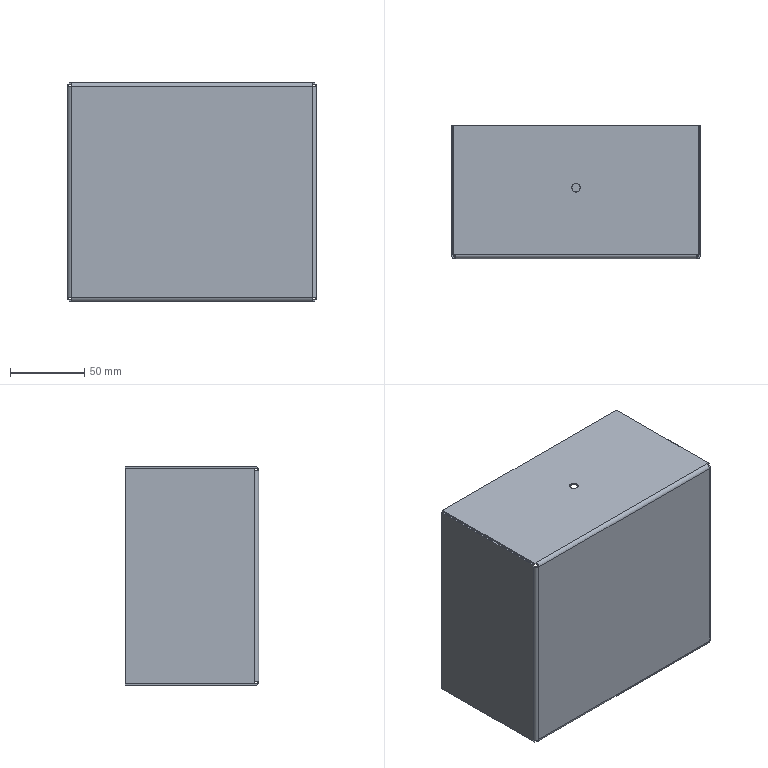Part | NX | 1 solid | 50 faces | box 167.7 x 90 x 147.4 mm | volume 79424 mm3 | plane 38 | cylinder 10 | cone 2 | commonest cylinder face diameters 3.2 x4 5.2 x4 5.5 x2
STEP:
#1=CARTESIAN_POINT('',(2221.7,-122.9,209.129));
#2=VERTEX_POINT('',#1);
#3=CARTESIAN_POINT('',(2221.7,-35.5,209.129));
#4=VERTEX_POINT('',#3);
#5=CARTESIAN_POINT('',(2221.7,-124.5,209.129));
#6=DIRECTION('',(0.,1.,0.));
#7=VECTOR('',#6,1000.);
#8=LINE('',#5,#7);
#9=EDGE_CURVE('',#2,#4,#8,.T.);
#10=ORIENTED_EDGE('',*,*,#9,.F.);
#11=CARTESIAN_POINT('',(2221.7,-122.9,207.6));
#12=VERTEX_POINT('',#11);
#13=CARTESIAN_POINT('',(2221.7,-122.9,119.504));
#14=DIRECTION('',(0.,0.,1.));
#15=VECTOR('',#14,1000.);
#16=LINE('',#13,#15);
#17=EDGE_CURVE('',#12,#2,#16,.T.);
#18=ORIENTED_EDGE('',*,*,#17,.F.);
#19=CARTESIAN_POINT('',(2221.7,-122.9,65.4));
#20=VERTEX_POINT('',#19);
#21=CARTESIAN_POINT('',(2221.7,-122.9,119.504));
#22=DIRECTION('',(0.,0.,1.));
#23=VECTOR('',#22,1000.);
#24=LINE('',#21,#23);
#25=EDGE_CURVE('',#20,#12,#24,.T.);
#26=ORIENTED_EDGE('',*,*,#25,.F.);
#27=CARTESIAN_POINT('',(2221.7,-122.9,63.871));
#28=VERTEX_POINT('',#27);
#29=CARTESIAN_POINT('',(2221.7,-122.9,119.504));
#30=DIRECTION('',(0.,0.,1.));
#31=VECTOR('',#30,1000.);
#32=LINE('',#29,#31);
#33=EDGE_CURVE('',#28,#20,#32,.T.);
#34=ORIENTED_EDGE('',*,*,#33,.F.);
#35=CARTESIAN_POINT('',(2221.7,-35.5,63.871));
#36=VERTEX_POINT('',#35);
#37=CARTESIAN_POINT('',(2221.7,-124.5,63.871));
#38=DIRECTION('',(0.,-1.,0.));
#39=VECTOR('',#38,1000.);
#40=LINE('',#37,#39);
#41=EDGE_CURVE('',#36,#28,#40,.T.);
#42=ORIENTED_EDGE('',*,*,#41,.F.);
#43=CARTESIAN_POINT('',(2221.7,-35.5,119.504));
#44=DIRECTION('',(0.,0.,-1.));
#45=VECTOR('',#44,1000.);
#46=LINE('',#43,#45);
#47=EDGE_CURVE('',#4,#36,#46,.T.);
#48=ORIENTED_EDGE('',*,*,#47,.F.);
#49=EDGE_LOOP('',(#10,#18,#26,#34,#42,#48));
#50=FACE_BOUND('',#49,.T.);
#51=CARTESIAN_POINT('',(2221.7,-188.294,119.504));
#52=DIRECTION('',(-1.,0.,0.));
#53=DIRECTION('',(0.,0.,1.));
#54=AXIS2_PLACEMENT_3D('',#51,#52,#53);
#55=PLANE('',#54);
#56=ADVANCED_FACE('',(#50),#55,.F.);
#57=CARTESIAN_POINT('',(2056.6,-122.9,62.8));
#58=VERTEX_POINT('',#57);
#59=CARTESIAN_POINT('',(2219.1,-122.9,62.8));
#60=VERTEX_POINT('',#59);
#61=CARTESIAN_POINT('',(2156.806,-122.9,62.8));
#62=DIRECTION('',(1.,0.,0.));
#63=VECTOR('',#62,1000.);
#64=LINE('',#61,#63);
#65=EDGE_CURVE('',#58,#60,#64,.T.);
#66=ORIENTED_EDGE('',*,*,#65,.F.);
#67=CARTESIAN_POINT('',(2055.071,-122.9,62.8));
#68=VERTEX_POINT('',#67);
#69=CARTESIAN_POINT('',(2156.806,-122.9,62.8));
#70=DIRECTION('',(1.,0.,0.));
#71=VECTOR('',#70,1000.);
#72=LINE('',#69,#71);
#73=EDGE_CURVE('',#68,#58,#72,.T.);
#74=ORIENTED_EDGE('',*,*,#73,.F.);
#75=CARTESIAN_POINT('',(2055.071,-35.5,62.8));
#76=VERTEX_POINT('',#75);
#77=CARTESIAN_POINT('',(2055.071,-124.5,62.8));
#78=DIRECTION('',(0.,-1.,0.));
#79=VECTOR('',#78,1000.);
#80=LINE('',#77,#79);
#81=EDGE_CURVE('',#76,#68,#80,.T.);
#82=ORIENTED_EDGE('',*,*,#81,.F.);
#83=CARTESIAN_POINT('',(2220.629,-35.5,62.8));
#84=VERTEX_POINT('',#83);
#85=CARTESIAN_POINT('',(2156.806,-35.5,62.8));
#86=DIRECTION('',(-1.,0.,0.));
#87=VECTOR('',#86,1000.);
#88=LINE('',#85,#87);
#89=EDGE_CURVE('',#84,#76,#88,.T.);
#90=ORIENTED_EDGE('',*,*,#89,.F.);
#91=CARTESIAN_POINT('',(2220.629,-122.9,62.8));
#92=VERTEX_POINT('',#91);
#93=CARTESIAN_POINT('',(2220.629,-124.5,62.8));
#94=DIRECTION('',(0.,1.,0.));
#95=VECTOR('',#94,1000.);
#96=LINE('',#93,#95);
#97=EDGE_CURVE('',#92,#84,#96,.T.);
#98=ORIENTED_EDGE('',*,*,#97,.F.);
#99=CARTESIAN_POINT('',(2156.806,-122.9,62.8));
#100=DIRECTION('',(1.,0.,0.));
#101=VECTOR('',#100,1000.);
#102=LINE('',#99,#101);
#103=EDGE_CURVE('',#60,#92,#102,.T.);
#104=ORIENTED_EDGE('',*,*,#103,.F.);
#105=EDGE_LOOP('',(#66,#74,#82,#90,#98,#104));
#106=FACE_BOUND('',#105,.T.);
#107=CARTESIAN_POINT('',(2156.806,-180.104,62.8));
#108=DIRECTION('',(0.,0.,1.));
#109=DIRECTION('',(1.,0.,0.));
#110=AXIS2_PLACEMENT_3D('',#107,#108,#109);
#111=PLANE('',#110);
#112=ADVANCED_FACE('',(#106),#111,.F.);
#113=CARTESIAN_POINT('',(2219.1,-125.5,207.6));
#114=VERTEX_POINT('',#113);
#115=CARTESIAN_POINT('',(2219.1,-122.9,207.6));
#116=DIRECTION('',(0.,0.,-1.));
#117=DIRECTION('',(1.,0.,0.));
#118=AXIS2_PLACEMENT_3D('',#115,#116,#117);
#119=CIRCLE('',#118,2.6);
#120=EDGE_CURVE('',#12,#114,#119,.T.);
#121=ORIENTED_EDGE('',*,*,#120,.T.);
#122=CARTESIAN_POINT('',(2219.1,-125.5,65.4));
#123=VERTEX_POINT('',#122);
#124=CARTESIAN_POINT('',(2219.1,-125.5,119.504));
#125=DIRECTION('',(0.,0.,1.));
#126=VECTOR('',#125,1000.);
#127=LINE('',#124,#126);
#128=EDGE_CURVE('',#123,#114,#127,.T.);
#129=ORIENTED_EDGE('',*,*,#128,.F.);
#130=CARTESIAN_POINT('',(2219.1,-122.9,65.4));
#131=DIRECTION('',(0.,0.,1.));
#132=DIRECTION('',(0.,-1.,0.));
#133=AXIS2_PLACEMENT_3D('',#130,#131,#132);
#134=CIRCLE('',#133,2.6);
#135=EDGE_CURVE('',#123,#20,#134,.T.);
#136=ORIENTED_EDGE('',*,*,#135,.T.);
#137=ORIENTED_EDGE('',*,*,#25,.T.);
#138=EDGE_LOOP('',(#121,#129,#136,#137));
#139=FACE_BOUND('',#138,.T.);
#140=CARTESIAN_POINT('',(2219.1,-122.9,65.4));
#141=DIRECTION('',(0.,0.,-1.));
#142=DIRECTION('',(1.,0.,0.));
#143=AXIS2_PLACEMENT_3D('',#140,#141,#142);
#144=CYLINDRICAL_SURFACE('',#143,2.6);
#145=ADVANCED_FACE('',(#139),#144,.T.);
#146=CARTESIAN_POINT('',(2054.,-122.9,65.4));
#147=VERTEX_POINT('',#146);
#148=CARTESIAN_POINT('',(2056.6,-125.5,65.4));
#149=VERTEX_POINT('',#148);
#150=CARTESIAN_POINT('',(2056.6,-122.9,65.4));
#151=DIRECTION('',(0.,0.,1.));
#152=DIRECTION('',(-1.,0.,0.));
#153=AXIS2_PLACEMENT_3D('',#150,#151,#152);
#154=CIRCLE('',#153,2.6);
#155=EDGE_CURVE('',#147,#149,#154,.T.);
#156=ORIENTED_EDGE('',*,*,#155,.T.);
#157=CARTESIAN_POINT('',(2056.6,-125.5,207.6));
#158=VERTEX_POINT('',#157);
#159=CARTESIAN_POINT('',(2056.6,-125.5,119.504));
#160=DIRECTION('',(0.,0.,-1.));
#161=VECTOR('',#160,1000.);
#162=LINE('',#159,#161);
#163=EDGE_CURVE('',#158,#149,#162,.T.);
#164=ORIENTED_EDGE('',*,*,#163,.F.);
#165=CARTESIAN_POINT('',(2054.,-122.9,207.6));
#166=VERTEX_POINT('',#165);
#167=CARTESIAN_POINT('',(2056.6,-122.9,207.6));
#168=DIRECTION('',(0.,0.,-1.));
#169=DIRECTION('',(0.,-1.,0.));
#170=AXIS2_PLACEMENT_3D('',#167,#168,#169);
#171=CIRCLE('',#170,2.6);
#172=EDGE_CURVE('',#158,#166,#171,.T.);
#173=ORIENTED_EDGE('',*,*,#172,.T.);
#174=CARTESIAN_POINT('',(2054.,-122.9,119.504));
#175=DIRECTION('',(0.,0.,-1.));
#176=VECTOR('',#175,1000.);
#177=LINE('',#174,#176);
#178=EDGE_CURVE('',#166,#147,#177,.T.);
#179=ORIENTED_EDGE('',*,*,#178,.T.);
#180=EDGE_LOOP('',(#156,#164,#173,#179));
#181=FACE_BOUND('',#180,.T.);
#182=CARTESIAN_POINT('',(2056.6,-122.9,207.6));
#183=DIRECTION('',(0.,0.,1.));
#184=DIRECTION('',(-1.,0.,0.));
#185=AXIS2_PLACEMENT_3D('',#182,#183,#184);
#186=CYLINDRICAL_SURFACE('',#185,2.6);
#187=ADVANCED_FACE('',(#181),#186,.T.);
#188=CARTESIAN_POINT('',(2054.,-122.9,63.871));
#189=VERTEX_POINT('',#188);
#190=CARTESIAN_POINT('',(2054.,-122.9,119.504));
#191=DIRECTION('',(0.,0.,1.));
#192=VECTOR('',#191,1000.);
#193=LINE('',#190,#192);
#194=EDGE_CURVE('',#189,#147,#193,.T.);
#195=ORIENTED_EDGE('',*,*,#194,.T.);
#196=ORIENTED_EDGE('',*,*,#178,.F.);
#197=CARTESIAN_POINT('',(2054.,-122.9,209.129));
#198=VERTEX_POINT('',#197);
#199=CARTESIAN_POINT('',(2054.,-122.9,119.504));
#200=DIRECTION('',(0.,0.,1.));
#201=VECTOR('',#200,1000.);
#202=LINE('',#199,#201);
#203=EDGE_CURVE('',#166,#198,#202,.T.);
#204=ORIENTED_EDGE('',*,*,#203,.T.);
#205=CARTESIAN_POINT('',(2054.,-35.5,209.129));
#206=VERTEX_POINT('',#205);
#207=CARTESIAN_POINT('',(2054.,-124.5,209.129));
#208=DIRECTION('',(0.,-1.,0.));
#209=VECTOR('',#208,1000.);
#210=LINE('',#207,#209);
#211=EDGE_CURVE('',#206,#198,#210,.T.);
#212=ORIENTED_EDGE('',*,*,#211,.F.);
#213=CARTESIAN_POINT('',(2054.,-35.5,63.871));
#214=VERTEX_POINT('',#213);
#215=CARTESIAN_POINT('',(2054.,-35.5,119.504));
#216=DIRECTION('',(0.,0.,1.));
#217=VECTOR('',#216,1000.);
#218=LINE('',#215,#217);
#219=EDGE_CURVE('',#214,#206,#218,.T.);
#220=ORIENTED_EDGE('',*,*,#219,.F.);
#221=CARTESIAN_POINT('',(2054.,-124.5,63.871));
#222=DIRECTION('',(0.,1.,0.));
#223=VECTOR('',#222,1000.);
#224=LINE('',#221,#223);
#225=EDGE_CURVE('',#189,#214,#224,.T.);
#226=ORIENTED_EDGE('',*,*,#225,.F.);
#227=EDGE_LOOP('',(#195,#196,#204,#212,#220,#226));
#228=FACE_BOUND('',#227,.T.);
#229=CARTESIAN_POINT('',(2054.,-226.206,119.504));
#230=DIRECTION('',(1.,0.,0.));
#231=DIRECTION('',(0.,1.,0.));
#232=AXIS2_PLACEMENT_3D('',#229,#230,#231);
#233=PLANE('',#232);
#234=ADVANCED_FACE('',(#228),#233,.F.);
#235=CARTESIAN_POINT('',(2156.806,-125.5,65.4));
#236=DIRECTION('',(1.,0.,0.));
#237=VECTOR('',#236,1000.);
#238=LINE('',#235,#237);
#239=EDGE_CURVE('',#149,#123,#238,.T.);
#240=ORIENTED_EDGE('',*,*,#239,.F.);
#241=CARTESIAN_POINT('',(2056.6,-122.9,65.4));
#242=DIRECTION('',(-1.,0.,0.));
#243=DIRECTION('',(0.,0.,-1.));
#244=AXIS2_PLACEMENT_3D('',#241,#242,#243);
#245=CIRCLE('',#244,2.6);
#246=EDGE_CURVE('',#58,#149,#245,.T.);
#247=ORIENTED_EDGE('',*,*,#246,.F.);
#248=ORIENTED_EDGE('',*,*,#65,.T.);
#249=CARTESIAN_POINT('',(2219.1,-122.9,65.4));
#250=DIRECTION('',(-1.,0.,0.));
#251=DIRECTION('',(0.,0.,-1.));
#252=AXIS2_PLACEMENT_3D('',#249,#250,#251);
#253=CIRCLE('',#252,2.6);
#254=EDGE_CURVE('',#60,#123,#253,.T.);
#255=ORIENTED_EDGE('',*,*,#254,.T.);
#256=EDGE_LOOP('',(#240,#247,#248,#255));
#257=FACE_BOUND('',#256,.T.);
#258=CARTESIAN_POINT('',(2056.6,-122.9,65.4));
#259=DIRECTION('',(-1.,0.,0.));
#260=DIRECTION('',(0.,0.,-1.));
#261=AXIS2_PLACEMENT_3D('',#258,#259,#260);
#262=CYLINDRICAL_SURFACE('',#261,2.6);
#263=ADVANCED_FACE('',(#257),#262,.T.);
#264=CARTESIAN_POINT('',(2220.7,-122.9,65.4));
#265=VERTEX_POINT('',#264);
#266=CARTESIAN_POINT('',(2219.1,-124.5,65.4));
#267=VERTEX_POINT('',#266);
#268=CARTESIAN_POINT('',(2219.1,-122.9,65.4));
#269=DIRECTION('',(0.,0.,-1.));
#270=DIRECTION('',(1.,0.,0.));
#271=AXIS2_PLACEMENT_3D('',#268,#269,#270);
#272=CIRCLE('',#271,1.6);
#273=EDGE_CURVE('',#265,#267,#272,.T.);
#274=ORIENTED_EDGE('',*,*,#273,.T.);
#275=CARTESIAN_POINT('',(2219.1,-124.5,207.6));
#276=VERTEX_POINT('',#275);
#277=CARTESIAN_POINT('',(2219.1,-124.5,119.504));
#278=DIRECTION('',(0.,0.,-1.));
#279=VECTOR('',#278,1000.);
#280=LINE('',#277,#279);
#281=EDGE_CURVE('',#276,#267,#280,.T.);
#282=ORIENTED_EDGE('',*,*,#281,.F.);
#283=CARTESIAN_POINT('',(2220.7,-122.9,207.6));
#284=VERTEX_POINT('',#283);
#285=CARTESIAN_POINT('',(2219.1,-122.9,207.6));
#286=DIRECTION('',(0.,0.,1.));
#287=DIRECTION('',(0.,-1.,0.));
#288=AXIS2_PLACEMENT_3D('',#285,#286,#287);
#289=CIRCLE('',#288,1.6);
#290=EDGE_CURVE('',#276,#284,#289,.T.);
#291=ORIENTED_EDGE('',*,*,#290,.T.);
#292=CARTESIAN_POINT('',(2220.7,-122.9,119.504));
#293=DIRECTION('',(0.,0.,-1.));
#294=VECTOR('',#293,1000.);
#295=LINE('',#292,#294);
#296=EDGE_CURVE('',#284,#265,#295,.T.);
#297=ORIENTED_EDGE('',*,*,#296,.T.);
#298=EDGE_LOOP('',(#274,#282,#291,#297));
#299=FACE_BOUND('',#298,.T.);
#300=CARTESIAN_POINT('',(2219.1,-122.9,65.4));
#301=DIRECTION('',(0.,0.,-1.));
#302=DIRECTION('',(1.,0.,0.));
#303=AXIS2_PLACEMENT_3D('',#300,#301,#302);
#304=CYLINDRICAL_SURFACE('',#303,1.6);
#305=ADVANCED_FACE('',(#299),#304,.F.);
#306=ORIENTED_EDGE('',*,*,#47,.T.);
#307=CARTESIAN_POINT('',(2220.7,-35.5,63.871));
#308=VERTEX_POINT('',#307);
#309=CARTESIAN_POINT('',(2156.806,-35.5,63.871));
#310=DIRECTION('',(1.,0.,0.));
#311=VECTOR('',#310,1000.);
#312=LINE('',#309,#311);
#313=EDGE_CURVE('',#308,#36,#312,.T.);
#314=ORIENTED_EDGE('',*,*,#313,.F.);
#315=CARTESIAN_POINT('',(2220.7,-35.5,209.129));
#316=VERTEX_POINT('',#315);
#317=CARTESIAN_POINT('',(2220.7,-35.5,119.504));
#318=DIRECTION('',(0.,0.,1.));
#319=VECTOR('',#318,1000.);
#320=LINE('',#317,#319);
#321=EDGE_CURVE('',#308,#316,#320,.T.);
#322=ORIENTED_EDGE('',*,*,#321,.T.);
#323=CARTESIAN_POINT('',(2156.806,-35.5,209.129));
#324=DIRECTION('',(-1.,0.,0.));
#325=VECTOR('',#324,1000.);
#326=LINE('',#323,#325);
#327=EDGE_CURVE('',#4,#316,#326,.T.);
#328=ORIENTED_EDGE('',*,*,#327,.F.);
#329=EDGE_LOOP('',(#306,#314,#322,#328));
#330=FACE_BOUND('',#329,.T.);
#331=CARTESIAN_POINT('',(2221.7,-35.5,62.8));
#332=DIRECTION('',(0.,1.,0.));
#333=DIRECTION('',(1.,0.,0.));
#334=AXIS2_PLACEMENT_3D('',#331,#332,#333);
#335=PLANE('',#334);
#336=ADVANCED_FACE('',(#330),#335,.T.);
#337=CARTESIAN_POINT('',(2220.7,-122.9,209.129));
#338=VERTEX_POINT('',#337);
#339=CARTESIAN_POINT('',(2220.7,-124.5,209.129));
#340=DIRECTION('',(0.,-1.,0.));
#341=VECTOR('',#340,1000.);
#342=LINE('',#339,#341);
#343=EDGE_CURVE('',#316,#338,#342,.T.);
#344=ORIENTED_EDGE('',*,*,#343,.F.);
#345=ORIENTED_EDGE('',*,*,#321,.F.);
#346=CARTESIAN_POINT('',(2220.7,-122.9,63.871));
#347=VERTEX_POINT('',#346);
#348=CARTESIAN_POINT('',(2220.7,-124.5,63.871));
#349=DIRECTION('',(0.,1.,0.));
#350=VECTOR('',#349,1000.);
#351=LINE('',#348,#350);
#352=EDGE_CURVE('',#347,#308,#351,.T.);
#353=ORIENTED_EDGE('',*,*,#352,.F.);
#354=CARTESIAN_POINT('',(2220.7,-122.9,119.504));
#355=DIRECTION('',(0.,0.,1.));
#356=VECTOR('',#355,1000.);
#357=LINE('',#354,#356);
#358=EDGE_CURVE('',#347,#265,#357,.T.);
#359=ORIENTED_EDGE('',*,*,#358,.T.);
#360=ORIENTED_EDGE('',*,*,#296,.F.);
#361=CARTESIAN_POINT('',(2220.7,-122.9,119.504));
#362=DIRECTION('',(0.,0.,1.));
#363=VECTOR('',#362,1000.);
#364=LINE('',#361,#363);
#365=EDGE_CURVE('',#284,#338,#364,.T.);
#366=ORIENTED_EDGE('',*,*,#365,.T.);
#367=EDGE_LOOP('',(#344,#345,#353,#359,#360,#366));
#368=FACE_BOUND('',#367,.T.);
#369=CARTESIAN_POINT('',(2220.7,-123.4,210.2));
#370=DIRECTION('',(1.,0.,0.));
#371=DIRECTION('',(0.,1.,0.));
#372=AXIS2_PLACEMENT_3D('',#369,#370,#371);
#373=PLANE('',#372);
#374=ADVANCED_FACE('',(#368),#373,.F.);
#375=ORIENTED_EDGE('',*,*,#225,.T.);
#376=CARTESIAN_POINT('',(2055.,-35.5,63.871));
#377=VERTEX_POINT('',#376);
#378=CARTESIAN_POINT('',(2156.806,-35.5,63.871));
#379=DIRECTION('',(1.,0.,0.));
#380=VECTOR('',#379,1000.);
#381=LINE('',#378,#380);
#382=EDGE_CURVE('',#214,#377,#381,.T.);
#383=ORIENTED_EDGE('',*,*,#382,.T.);
#384=CARTESIAN_POINT('',(2055.,-122.9,63.871));
#385=VERTEX_POINT('',#384);
#386=CARTESIAN_POINT('',(2055.,-124.5,63.871));
#387=DIRECTION('',(0.,-1.,0.));
#388=VECTOR('',#387,1000.);
#389=LINE('',#386,#388);
#390=EDGE_CURVE('',#377,#385,#389,.T.);
#391=ORIENTED_EDGE('',*,*,#390,.T.);
#392=CARTESIAN_POINT('',(2055.,-122.9,63.871));
#393=DIRECTION('',(-1.,0.,0.));
#394=VECTOR('',#393,1000.);
#395=LINE('',#392,#394);
#396=EDGE_CURVE('',#385,#189,#395,.T.);
#397=ORIENTED_EDGE('',*,*,#396,.T.);
#398=EDGE_LOOP('',(#375,#383,#391,#397));
#399=FACE_BOUND('',#398,.T.);
#400=CARTESIAN_POINT('',(2055.,-64.2,63.871));
#401=DIRECTION('',(0.,0.,-1.));
#402=DIRECTION('',(0.,-1.,0.));
#403=AXIS2_PLACEMENT_3D('',#400,#401,#402);
#404=PLANE('',#403);
#405=ADVANCED_FACE('',(#399),#404,.T.);
#406=CARTESIAN_POINT('',(2055.,-122.9,207.6));
#407=VERTEX_POINT('',#406);
#408=CARTESIAN_POINT('',(2056.6,-124.5,207.6));
#409=VERTEX_POINT('',#408);
#410=CARTESIAN_POINT('',(2056.6,-122.9,207.6));
#411=DIRECTION('',(0.,0.,1.));
#412=DIRECTION('',(-1.,0.,0.));
#413=AXIS2_PLACEMENT_3D('',#410,#411,#412);
#414=CIRCLE('',#413,1.6);
#415=EDGE_CURVE('',#407,#409,#414,.T.);
#416=ORIENTED_EDGE('',*,*,#415,.T.);
#417=CARTESIAN_POINT('',(2056.6,-124.5,65.4));
#418=VERTEX_POINT('',#417);
#419=CARTESIAN_POINT('',(2056.6,-124.5,119.504));
#420=DIRECTION('',(0.,0.,1.));
#421=VECTOR('',#420,1000.);
#422=LINE('',#419,#421);
#423=EDGE_CURVE('',#418,#409,#422,.T.);
#424=ORIENTED_EDGE('',*,*,#423,.F.);
#425=CARTESIAN_POINT('',(2055.,-122.9,65.4));
#426=VERTEX_POINT('',#425);
#427=CARTESIAN_POINT('',(2056.6,-122.9,65.4));
#428=DIRECTION('',(0.,0.,-1.));
#429=DIRECTION('',(0.,-1.,0.));
#430=AXIS2_PLACEMENT_3D('',#427,#428,#429);
#431=CIRCLE('',#430,1.6);
#432=EDGE_CURVE('',#418,#426,#431,.T.);
#433=ORIENTED_EDGE('',*,*,#432,.T.);
#434=CARTESIAN_POINT('',(2055.,-122.9,119.504));
#435=DIRECTION('',(0.,0.,1.));
#436=VECTOR('',#435,1000.);
#437=LINE('',#434,#436);
#438=EDGE_CURVE('',#426,#407,#437,.T.);
#439=ORIENTED_EDGE('',*,*,#438,.T.);
#440=EDGE_LOOP('',(#416,#424,#433,#439));
#441=FACE_BOUND('',#440,.T.);
#442=CARTESIAN_POINT('',(2056.6,-122.9,207.6));
#443=DIRECTION('',(0.,0.,1.));
#444=DIRECTION('',(-1.,0.,0.));
#445=AXIS2_PLACEMENT_3D('',#442,#443,#444);
#446=CYLINDRICAL_SURFACE('',#445,1.6);
#447=ADVANCED_FACE('',(#441),#446,.F.);
#448=ORIENTED_EDGE('',*,*,#390,.F.);
#449=CARTESIAN_POINT('',(2055.,-35.5,209.129));
#450=VERTEX_POINT('',#449);
#451=CARTESIAN_POINT('',(2055.,-35.5,119.504));
#452=DIRECTION('',(0.,0.,-1.));
#453=VECTOR('',#452,1000.);
#454=LINE('',#451,#453);
#455=EDGE_CURVE('',#450,#377,#454,.T.);
#456=ORIENTED_EDGE('',*,*,#455,.F.);
#457=CARTESIAN_POINT('',(2055.,-122.9,209.129));
#458=VERTEX_POINT('',#457);
#459=CARTESIAN_POINT('',(2055.,-124.5,209.129));
#460=DIRECTION('',(0.,1.,0.));
#461=VECTOR('',#460,1000.);
#462=LINE('',#459,#461);
#463=EDGE_CURVE('',#458,#450,#462,.T.);
#464=ORIENTED_EDGE('',*,*,#463,.F.);
#465=CARTESIAN_POINT('',(2055.,-122.9,119.504));
#466=DIRECTION('',(0.,0.,-1.));
#467=VECTOR('',#466,1000.);
#468=LINE('',#465,#467);
#469=EDGE_CURVE('',#458,#407,#468,.T.);
#470=ORIENTED_EDGE('',*,*,#469,.T.);
#471=ORIENTED_EDGE('',*,*,#438,.F.);
#472=CARTESIAN_POINT('',(2055.,-122.9,119.504));
#473=DIRECTION('',(0.,0.,-1.));
#474=VECTOR('',#473,1000.);
#475=LINE('',#472,#474);
#476=EDGE_CURVE('',#426,#385,#475,.T.);
#477=ORIENTED_EDGE('',*,*,#476,.T.);
#478=EDGE_LOOP('',(#448,#456,#464,#470,#471,#477));
#479=FACE_BOUND('',#478,.T.);
#480=CARTESIAN_POINT('',(2055.,-123.4,62.8));
#481=DIRECTION('',(-1.,0.,0.));
#482=DIRECTION('',(0.,0.,1.));
#483=AXIS2_PLACEMENT_3D('',#480,#481,#482);
#484=PLANE('',#483);
#485=ADVANCED_FACE('',(#479),#484,.F.);
#486=ORIENTED_EDGE('',*,*,#219,.T.);
#487=CARTESIAN_POINT('',(2156.806,-35.5,209.129));
#488=DIRECTION('',(-1.,0.,0.));
#489=VECTOR('',#488,1000.);
#490=LINE('',#487,#489);
#491=EDGE_CURVE('',#450,#206,#490,.T.);
#492=ORIENTED_EDGE('',*,*,#491,.F.);
#493=ORIENTED_EDGE('',*,*,#455,.T.);
#494=ORIENTED_EDGE('',*,*,#382,.F.);
#495=EDGE_LOOP('',(#486,#492,#493,#494));
#496=FACE_BOUND('',#495,.T.);
#497=CARTESIAN_POINT('',(2054.,-35.5,210.2));
#498=DIRECTION('',(0.,1.,0.));
#499=DIRECTION('',(1.,0.,0.));
#500=AXIS2_PLACEMENT_3D('',#497,#498,#499);
#501=PLANE('',#500);
#502=ADVANCED_FACE('',(#496),#501,.T.);
#503=CARTESIAN_POINT('',(2056.6,-122.9,209.2));
#504=VERTEX_POINT('',#503);
#505=CARTESIAN_POINT('',(2056.6,-122.9,207.6));
#506=DIRECTION('',(1.,0.,0.));
#507=DIRECTION('',(0.,0.,1.));
#508=AXIS2_PLACEMENT_3D('',#505,#506,#507);
#509=CIRCLE('',#508,1.6);
#510=EDGE_CURVE('',#504,#409,#509,.T.);
#511=ORIENTED_EDGE('',*,*,#510,.F.);
#512=CARTESIAN_POINT('',(2219.1,-122.9,209.2));
#513=VERTEX_POINT('',#512);
#514=CARTESIAN_POINT('',(2156.806,-122.9,209.2));
#515=DIRECTION('',(1.,0.,0.));
#516=VECTOR('',#515,1000.);
#517=LINE('',#514,#516);
#518=EDGE_CURVE('',#504,#513,#517,.T.);
#519=ORIENTED_EDGE('',*,*,#518,.T.);
#520=CARTESIAN_POINT('',(2219.1,-122.9,207.6));
#521=DIRECTION('',(-1.,0.,0.));
#522=DIRECTION('',(0.,-1.,0.));
#523=AXIS2_PLACEMENT_3D('',#520,#521,#522);
#524=CIRCLE('',#523,1.6);
#525=EDGE_CURVE('',#276,#513,#524,.T.);
#526=ORIENTED_EDGE('',*,*,#525,.F.);
#527=CARTESIAN_POINT('',(2156.806,-124.5,207.6));
#528=DIRECTION('',(1.,0.,0.));
#529=VECTOR('',#528,1000.);
#530=LINE('',#527,#529);
#531=EDGE_CURVE('',#409,#276,#530,.T.);
#532=ORIENTED_EDGE('',*,*,#531,.F.);
#533=EDGE_LOOP('',(#511,#519,#526,#532));
#534=FACE_BOUND('',#533,.T.);
#535=CARTESIAN_POINT('',(2219.1,-122.9,207.6));
#536=DIRECTION('',(1.,0.,0.));
#537=DIRECTION('',(0.,0.,1.));
#538=AXIS2_PLACEMENT_3D('',#535,#536,#537);
#539=CYLINDRICAL_SURFACE('',#538,1.6);
#540=ADVANCED_FACE('',(#534),#539,.F.);
#541=ORIENTED_EDGE('',*,*,#463,.T.);
#542=ORIENTED_EDGE('',*,*,#491,.T.);
#543=ORIENTED_EDGE('',*,*,#211,.T.);
#544=CARTESIAN_POINT('',(2055.,-122.9,209.129));
#545=DIRECTION('',(1.,0.,0.));
#546=VECTOR('',#545,1000.);
#547=LINE('',#544,#546);
#548=EDGE_CURVE('',#198,#458,#547,.T.);
#549=ORIENTED_EDGE('',*,*,#548,.T.);
#550=EDGE_LOOP('',(#541,#542,#543,#549));
#551=FACE_BOUND('',#550,.T.);
#552=CARTESIAN_POINT('',(2055.,-64.2,209.129));
#553=DIRECTION('',(0.,0.,1.));
#554=DIRECTION('',(1.,0.,0.));
#555=AXIS2_PLACEMENT_3D('',#552,#553,#554);
#556=PLANE('',#555);
#557=ADVANCED_FACE('',(#551),#556,.T.);
#558=CARTESIAN_POINT('',(2220.7,-122.9,63.871));
#559=DIRECTION('',(-1.,0.,0.));
#560=VECTOR('',#559,1000.);
#561=LINE('',#558,#560);
#562=EDGE_CURVE('',#28,#347,#561,.T.);
#563=ORIENTED_EDGE('',*,*,#562,.T.);
#564=ORIENTED_EDGE('',*,*,#352,.T.);
#565=ORIENTED_EDGE('',*,*,#313,.T.);
#566=ORIENTED_EDGE('',*,*,#41,.T.);
#567=EDGE_LOOP('',(#563,#564,#565,#566));
#568=FACE_BOUND('',#567,.T.);
#569=CARTESIAN_POINT('',(2220.7,-64.2,63.871));
#570=DIRECTION('',(0.,0.,-1.));
#571=DIRECTION('',(0.,-1.,0.));
#572=AXIS2_PLACEMENT_3D('',#569,#570,#571);
#573=PLANE('',#572);
#574=ADVANCED_FACE('',(#568),#573,.T.);
#575=ORIENTED_EDGE('',*,*,#33,.T.);
#576=CARTESIAN_POINT('',(2221.7,-122.9,65.4));
#577=DIRECTION('',(-1.,0.,0.));
#578=VECTOR('',#577,1000.);
#579=LINE('',#576,#578);
#580=EDGE_CURVE('',#20,#265,#579,.T.);
#581=ORIENTED_EDGE('',*,*,#580,.T.);
#582=ORIENTED_EDGE('',*,*,#358,.F.);
#583=ORIENTED_EDGE('',*,*,#562,.F.);
#584=EDGE_LOOP('',(#575,#581,#582,#583));
#585=FACE_BOUND('',#584,.T.);
#586=CARTESIAN_POINT('',(2221.7,-122.9,65.4));
#587=DIRECTION('',(0.,-1.,0.));
#588=DIRECTION('',(0.,0.,-1.));
#589=AXIS2_PLACEMENT_3D('',#586,#587,#588);
#590=PLANE('',#589);
#591=ADVANCED_FACE('',(#585),#590,.T.);
#592=ORIENTED_EDGE('',*,*,#135,.F.);
#593=CARTESIAN_POINT('',(2219.1,-125.5,65.4));
#594=DIRECTION('',(0.,1.,0.));
#595=VECTOR('',#594,1000.);
#596=LINE('',#593,#595);
#597=EDGE_CURVE('',#123,#267,#596,.T.);
#598=ORIENTED_EDGE('',*,*,#597,.T.);
#599=ORIENTED_EDGE('',*,*,#273,.F.);
#600=ORIENTED_EDGE('',*,*,#580,.F.);
#601=EDGE_LOOP('',(#592,#598,#599,#600));
#602=FACE_BOUND('',#601,.T.);
#603=CARTESIAN_POINT('',(2219.1,-122.9,65.4));
#604=DIRECTION('',(0.,0.,1.));
#605=DIRECTION('',(1.,0.,0.));
#606=AXIS2_PLACEMENT_3D('',#603,#604,#605);
#607=PLANE('',#606);
#608=ADVANCED_FACE('',(#602),#607,.F.);
#609=ORIENTED_EDGE('',*,*,#246,.T.);
#610=CARTESIAN_POINT('',(2056.6,-125.5,65.4));
#611=DIRECTION('',(0.,1.,0.));
#612=VECTOR('',#611,1000.);
#613=LINE('',#610,#612);
#614=EDGE_CURVE('',#149,#418,#613,.T.);
#615=ORIENTED_EDGE('',*,*,#614,.T.);
#616=CARTESIAN_POINT('',(2056.6,-122.9,63.8));
#617=VERTEX_POINT('',#616);
#618=CARTESIAN_POINT('',(2056.6,-122.9,65.4));
#619=DIRECTION('',(1.,0.,0.));
#620=DIRECTION('',(0.,-1.,0.));
#621=AXIS2_PLACEMENT_3D('',#618,#619,#620);
#622=CIRCLE('',#621,1.6);
#623=EDGE_CURVE('',#418,#617,#622,.T.);
#624=ORIENTED_EDGE('',*,*,#623,.T.);
#625=CARTESIAN_POINT('',(2056.6,-122.9,62.8));
#626=DIRECTION('',(0.,0.,1.));
#627=VECTOR('',#626,1000.);
#628=LINE('',#625,#627);
#629=EDGE_CURVE('',#58,#617,#628,.T.);
#630=ORIENTED_EDGE('',*,*,#629,.F.);
#631=EDGE_LOOP('',(#609,#615,#624,#630));
#632=FACE_BOUND('',#631,.T.);
#633=CARTESIAN_POINT('',(2056.6,-122.9,65.4));
#634=DIRECTION('',(-1.,0.,0.));
#635=DIRECTION('',(0.,1.,0.));
#636=AXIS2_PLACEMENT_3D('',#633,#634,#635);
#637=PLANE('',#636);
#638=ADVANCED_FACE('',(#632),#637,.T.);
#639=CARTESIAN_POINT('',(2156.806,-124.5,65.4));
#640=DIRECTION('',(-1.,0.,0.));
#641=VECTOR('',#640,1000.);
#642=LINE('',#639,#641);
#643=EDGE_CURVE('',#267,#418,#642,.T.);
#644=ORIENTED_EDGE('',*,*,#643,.F.);
#645=CARTESIAN_POINT('',(2219.1,-122.9,63.8));
#646=VERTEX_POINT('',#645);
#647=CARTESIAN_POINT('',(2219.1,-122.9,65.4));
#648=DIRECTION('',(-1.,0.,0.));
#649=DIRECTION('',(0.,0.,-1.));
#650=AXIS2_PLACEMENT_3D('',#647,#648,#649);
#651=CIRCLE('',#650,1.6);
#652=EDGE_CURVE('',#646,#267,#651,.T.);
#653=ORIENTED_EDGE('',*,*,#652,.F.);
#654=CARTESIAN_POINT('',(2156.806,-122.9,63.8));
#655=DIRECTION('',(-1.,0.,0.));
#656=VECTOR('',#655,1000.);
#657=LINE('',#654,#656);
#658=EDGE_CURVE('',#646,#617,#657,.T.);
#659=ORIENTED_EDGE('',*,*,#658,.T.);
#660=ORIENTED_EDGE('',*,*,#623,.F.);
#661=EDGE_LOOP('',(#644,#653,#659,#660));
#662=FACE_BOUND('',#661,.T.);
#663=CARTESIAN_POINT('',(2056.6,-122.9,65.4));
#664=DIRECTION('',(-1.,0.,0.));
#665=DIRECTION('',(0.,0.,-1.));
#666=AXIS2_PLACEMENT_3D('',#663,#664,#665);
#667=CYLINDRICAL_SURFACE('',#666,1.6);
#668=ADVANCED_FACE('',(#662),#667,.F.);
#669=ORIENTED_EDGE('',*,*,#658,.F.);
#670=CARTESIAN_POINT('',(2220.629,-122.9,63.8));
#671=VERTEX_POINT('',#670);
#672=CARTESIAN_POINT('',(2156.806,-122.9,63.8));
#673=DIRECTION('',(-1.,0.,0.));
#674=VECTOR('',#673,1000.);
#675=LINE('',#672,#674);
#676=EDGE_CURVE('',#671,#646,#675,.T.);
#677=ORIENTED_EDGE('',*,*,#676,.F.);
#678=CARTESIAN_POINT('',(2220.629,-35.5,63.8));
#679=VERTEX_POINT('',#678);
#680=CARTESIAN_POINT('',(2220.629,-124.5,63.8));
#681=DIRECTION('',(0.,1.,0.));
#682=VECTOR('',#681,1000.);
#683=LINE('',#680,#682);
#684=EDGE_CURVE('',#671,#679,#683,.T.);
#685=ORIENTED_EDGE('',*,*,#684,.T.);
#686=CARTESIAN_POINT('',(2055.071,-35.5,63.8));
#687=VERTEX_POINT('',#686);
#688=CARTESIAN_POINT('',(2156.806,-35.5,63.8));
#689=DIRECTION('',(1.,0.,0.));
#690=VECTOR('',#689,1000.);
#691=LINE('',#688,#690);
#692=EDGE_CURVE('',#687,#679,#691,.T.);
#693=ORIENTED_EDGE('',*,*,#692,.F.);
#694=CARTESIAN_POINT('',(2055.071,-122.9,63.8));
#695=VERTEX_POINT('',#694);
#696=CARTESIAN_POINT('',(2055.071,-124.5,63.8));
#697=DIRECTION('',(0.,-1.,0.));
#698=VECTOR('',#697,1000.);
#699=LINE('',#696,#698);
#700=EDGE_CURVE('',#687,#695,#699,.T.);
#701=ORIENTED_EDGE('',*,*,#700,.T.);
#702=CARTESIAN_POINT('',(2156.806,-122.9,63.8));
#703=DIRECTION('',(-1.,0.,0.));
#704=VECTOR('',#703,1000.);
#705=LINE('',#702,#704);
#706=EDGE_CURVE('',#617,#695,#705,.T.);
#707=ORIENTED_EDGE('',*,*,#706,.F.);
#708=EDGE_LOOP('',(#669,#677,#685,#693,#701,#707));
#709=FACE_BOUND('',#708,.T.);
#710=CARTESIAN_POINT('',(2054.,-123.4,63.8));
#711=DIRECTION('',(0.,0.,-1.));
#712=DIRECTION('',(-1.,0.,0.));
#713=AXIS2_PLACEMENT_3D('',#710,#711,#712);
#714=PLANE('',#713);
#715=ADVANCED_FACE('',(#709),#714,.F.);
#716=ORIENTED_EDGE('',*,*,#203,.F.);
#717=CARTESIAN_POINT('',(2054.,-122.9,207.6));
#718=DIRECTION('',(1.,0.,0.));
#719=VECTOR('',#718,1000.);
#720=LINE('',#717,#719);
#721=EDGE_CURVE('',#166,#407,#720,.T.);
#722=ORIENTED_EDGE('',*,*,#721,.T.);
#723=ORIENTED_EDGE('',*,*,#469,.F.);
#724=ORIENTED_EDGE('',*,*,#548,.F.);
#725=EDGE_LOOP('',(#716,#722,#723,#724));
#726=FACE_BOUND('',#725,.T.);
#727=CARTESIAN_POINT('',(2054.,-122.9,207.6));
#728=DIRECTION('',(0.,-1.,0.));
#729=DIRECTION('',(0.,0.,-1.));
#730=AXIS2_PLACEMENT_3D('',#727,#728,#729);
#731=PLANE('',#730);
#732=ADVANCED_FACE('',(#726),#731,.T.);
#733=CARTESIAN_POINT('',(2220.7,-122.9,209.129));
#734=DIRECTION('',(1.,0.,0.));
#735=VECTOR('',#734,1000.);
#736=LINE('',#733,#735);
#737=EDGE_CURVE('',#338,#2,#736,.T.);
#738=ORIENTED_EDGE('',*,*,#737,.T.);
#739=ORIENTED_EDGE('',*,*,#9,.T.);
#740=ORIENTED_EDGE('',*,*,#327,.T.);
#741=ORIENTED_EDGE('',*,*,#343,.T.);
#742=EDGE_LOOP('',(#738,#739,#740,#741));
#743=FACE_BOUND('',#742,.T.);
#744=CARTESIAN_POINT('',(2220.7,-64.2,209.129));
#745=DIRECTION('',(0.,0.,1.));
#746=DIRECTION('',(1.,0.,0.));
#747=AXIS2_PLACEMENT_3D('',#744,#745,#746);
#748=PLANE('',#747);
#749=ADVANCED_FACE('',(#743),#748,.T.);
#750=ORIENTED_EDGE('',*,*,#17,.T.);
#751=ORIENTED_EDGE('',*,*,#737,.F.);
#752=ORIENTED_EDGE('',*,*,#365,.F.);
#753=CARTESIAN_POINT('',(2221.7,-122.9,207.6));
#754=DIRECTION('',(-1.,0.,0.));
#755=VECTOR('',#754,1000.);
#756=LINE('',#753,#755);
#757=EDGE_CURVE('',#12,#284,#756,.T.);
#758=ORIENTED_EDGE('',*,*,#757,.F.);
#759=EDGE_LOOP('',(#750,#751,#752,#758));
#760=FACE_BOUND('',#759,.T.);
#761=CARTESIAN_POINT('',(2221.7,-122.9,210.7));
#762=DIRECTION('',(0.,-1.,0.));
#763=DIRECTION('',(0.,0.,-1.));
#764=AXIS2_PLACEMENT_3D('',#761,#762,#763);
#765=PLANE('',#764);
#766=ADVANCED_FACE('',(#760),#765,.T.);
#767=ORIENTED_EDGE('',*,*,#531,.T.);
#768=ORIENTED_EDGE('',*,*,#281,.T.);
#769=ORIENTED_EDGE('',*,*,#643,.T.);
#770=ORIENTED_EDGE('',*,*,#423,.T.);
#771=EDGE_LOOP('',(#767,#768,#769,#770));
#772=FACE_BOUND('',#771,.T.);
#773=CARTESIAN_POINT('',(2054.,-124.5,62.8));
#774=DIRECTION('',(0.,-1.,0.));
#775=DIRECTION('',(0.,0.,-1.));
#776=AXIS2_PLACEMENT_3D('',#773,#774,#775);
#777=PLANE('',#776);
#778=ADVANCED_FACE('',(#772),#777,.F.);
#779=ORIENTED_EDGE('',*,*,#518,.F.);
#780=CARTESIAN_POINT('',(2055.071,-122.9,209.2));
#781=VERTEX_POINT('',#780);
#782=CARTESIAN_POINT('',(2156.806,-122.9,209.2));
#783=DIRECTION('',(1.,0.,0.));
#784=VECTOR('',#783,1000.);
#785=LINE('',#782,#784);
#786=EDGE_CURVE('',#781,#504,#785,.T.);
#787=ORIENTED_EDGE('',*,*,#786,.F.);
#788=CARTESIAN_POINT('',(2055.071,-35.5,209.2));
#789=VERTEX_POINT('',#788);
#790=CARTESIAN_POINT('',(2055.071,-124.5,209.2));
#791=DIRECTION('',(0.,1.,0.));
#792=VECTOR('',#791,1000.);
#793=LINE('',#790,#792);
#794=EDGE_CURVE('',#781,#789,#793,.T.);
#795=ORIENTED_EDGE('',*,*,#794,.T.);
#796=CARTESIAN_POINT('',(2220.629,-35.5,209.2));
#797=VERTEX_POINT('',#796);
#798=CARTESIAN_POINT('',(2156.806,-35.5,209.2));
#799=DIRECTION('',(-1.,0.,0.));
#800=VECTOR('',#799,1000.);
#801=LINE('',#798,#800);
#802=EDGE_CURVE('',#797,#789,#801,.T.);
#803=ORIENTED_EDGE('',*,*,#802,.F.);
#804=CARTESIAN_POINT('',(2220.629,-122.9,209.2));
#805=VERTEX_POINT('',#804);
#806=CARTESIAN_POINT('',(2220.629,-124.5,209.2));
#807=DIRECTION('',(0.,-1.,0.));
#808=VECTOR('',#807,1000.);
#809=LINE('',#806,#808);
#810=EDGE_CURVE('',#797,#805,#809,.T.);
#811=ORIENTED_EDGE('',*,*,#810,.T.);
#812=CARTESIAN_POINT('',(2156.806,-122.9,209.2));
#813=DIRECTION('',(1.,0.,0.));
#814=VECTOR('',#813,1000.);
#815=LINE('',#812,#814);
#816=EDGE_CURVE('',#513,#805,#815,.T.);
#817=ORIENTED_EDGE('',*,*,#816,.F.);
#818=EDGE_LOOP('',(#779,#787,#795,#803,#811,#817));
#819=FACE_BOUND('',#818,.T.);
#820=CARTESIAN_POINT('',(2140.6,-77.765,209.2));
#821=VERTEX_POINT('',#820);
#822=CARTESIAN_POINT('',(2135.1,-77.765,209.2));
#823=VERTEX_POINT('',#822);
#824=CARTESIAN_POINT('',(2137.85,-77.765,209.2));
#825=DIRECTION('',(0.,0.,1.));
#826=DIRECTION('',(-1.,0.,0.));
#827=AXIS2_PLACEMENT_3D('',#824,#825,#826);
#828=CIRCLE('',#827,2.75);
#829=EDGE_CURVE('',#821,#823,#828,.T.);
#830=ORIENTED_EDGE('',*,*,#829,.T.);
#831=CARTESIAN_POINT('',(2137.85,-77.765,209.2));
#832=DIRECTION('',(0.,0.,1.));
#833=DIRECTION('',(-1.,0.,0.));
#834=AXIS2_PLACEMENT_3D('',#831,#832,#833);
#835=CIRCLE('',#834,2.75);
#836=EDGE_CURVE('',#823,#821,#835,.T.);
#837=ORIENTED_EDGE('',*,*,#836,.T.);
#838=EDGE_LOOP('',(#830,#837));
#839=FACE_BOUND('',#838,.T.);
#840=CARTESIAN_POINT('',(2054.,-270.8,209.2));
#841=DIRECTION('',(0.,0.,1.));
#842=DIRECTION('',(1.,0.,0.));
#843=AXIS2_PLACEMENT_3D('',#840,#841,#842);
#844=PLANE('',#843);
#845=ADVANCED_FACE('',(#819,#839),#844,.F.);
#846=ORIENTED_EDGE('',*,*,#97,.T.);
#847=CARTESIAN_POINT('',(2220.629,-35.5,119.504));
#848=DIRECTION('',(0.,0.,1.));
#849=VECTOR('',#848,1000.);
#850=LINE('',#847,#849);
#851=EDGE_CURVE('',#84,#679,#850,.T.);
#852=ORIENTED_EDGE('',*,*,#851,.T.);
#853=ORIENTED_EDGE('',*,*,#684,.F.);
#854=CARTESIAN_POINT('',(2220.629,-122.9,63.8));
#855=DIRECTION('',(0.,0.,-1.));
#856=VECTOR('',#855,1000.);
#857=LINE('',#854,#856);
#858=EDGE_CURVE('',#671,#92,#857,.T.);
#859=ORIENTED_EDGE('',*,*,#858,.T.);
#860=EDGE_LOOP('',(#846,#852,#853,#859));
#861=FACE_BOUND('',#860,.T.);
#862=CARTESIAN_POINT('',(2220.629,-25.5,62.8));
#863=DIRECTION('',(1.,0.,0.));
#864=DIRECTION('',(0.,1.,0.));
#865=AXIS2_PLACEMENT_3D('',#862,#863,#864);
#866=PLANE('',#865);
#867=ADVANCED_FACE('',(#861),#866,.T.);
#868=ORIENTED_EDGE('',*,*,#254,.F.);
#869=CARTESIAN_POINT('',(2219.1,-122.9,62.8));
#870=DIRECTION('',(0.,0.,1.));
#871=VECTOR('',#870,1000.);
#872=LINE('',#869,#871);
#873=EDGE_CURVE('',#60,#646,#872,.T.);
#874=ORIENTED_EDGE('',*,*,#873,.T.);
#875=ORIENTED_EDGE('',*,*,#652,.T.);
#876=ORIENTED_EDGE('',*,*,#597,.F.);
#877=EDGE_LOOP('',(#868,#874,#875,#876));
#878=FACE_BOUND('',#877,.T.);
#879=CARTESIAN_POINT('',(2219.1,-122.9,65.4));
#880=DIRECTION('',(-1.,0.,0.));
#881=DIRECTION('',(0.,1.,0.));
#882=AXIS2_PLACEMENT_3D('',#879,#880,#881);
#883=PLANE('',#882);
#884=ADVANCED_FACE('',(#878),#883,.F.);
#885=ORIENTED_EDGE('',*,*,#194,.F.);
#886=ORIENTED_EDGE('',*,*,#396,.F.);
#887=ORIENTED_EDGE('',*,*,#476,.F.);
#888=CARTESIAN_POINT('',(2054.,-122.9,65.4));
#889=DIRECTION('',(1.,0.,0.));
#890=VECTOR('',#889,1000.);
#891=LINE('',#888,#890);
#892=EDGE_CURVE('',#147,#426,#891,.T.);
#893=ORIENTED_EDGE('',*,*,#892,.F.);
#894=EDGE_LOOP('',(#885,#886,#887,#893));
#895=FACE_BOUND('',#894,.T.);
#896=CARTESIAN_POINT('',(2054.,-122.9,62.3));
#897=DIRECTION('',(0.,-1.,0.));
#898=DIRECTION('',(-1.,0.,0.));
#899=AXIS2_PLACEMENT_3D('',#896,#897,#898);
#900=PLANE('',#899);
#901=ADVANCED_FACE('',(#895),#900,.T.);
#902=CARTESIAN_POINT('',(2055.071,-122.9,63.8));
#903=DIRECTION('',(0.,0.,1.));
#904=VECTOR('',#903,1000.);
#905=LINE('',#902,#904);
#906=EDGE_CURVE('',#68,#695,#905,.T.);
#907=ORIENTED_EDGE('',*,*,#906,.T.);
#908=ORIENTED_EDGE('',*,*,#700,.F.);
#909=CARTESIAN_POINT('',(2055.071,-35.5,119.504));
#910=DIRECTION('',(0.,0.,-1.));
#911=VECTOR('',#910,1000.);
#912=LINE('',#909,#911);
#913=EDGE_CURVE('',#687,#76,#912,.T.);
#914=ORIENTED_EDGE('',*,*,#913,.T.);
#915=ORIENTED_EDGE('',*,*,#81,.T.);
#916=EDGE_LOOP('',(#907,#908,#914,#915));
#917=FACE_BOUND('',#916,.T.);
#918=CARTESIAN_POINT('',(2055.071,-123.4,62.8));
#919=DIRECTION('',(-1.,0.,0.));
#920=DIRECTION('',(0.,1.,0.));
#921=AXIS2_PLACEMENT_3D('',#918,#919,#920);
#922=PLANE('',#921);
#923=ADVANCED_FACE('',(#917),#922,.T.);
#924=ORIENTED_EDGE('',*,*,#89,.T.);
#925=ORIENTED_EDGE('',*,*,#913,.F.);
#926=ORIENTED_EDGE('',*,*,#692,.T.);
#927=ORIENTED_EDGE('',*,*,#851,.F.);
#928=EDGE_LOOP('',(#924,#925,#926,#927));
#929=FACE_BOUND('',#928,.T.);
#930=CARTESIAN_POINT('',(2055.071,-35.5,62.8));
#931=DIRECTION('',(0.,1.,0.));
#932=DIRECTION('',(1.,0.,0.));
#933=AXIS2_PLACEMENT_3D('',#930,#931,#932);
#934=PLANE('',#933);
#935=ADVANCED_FACE('',(#929),#934,.T.);
#936=ORIENTED_EDGE('',*,*,#858,.F.);
#937=ORIENTED_EDGE('',*,*,#676,.T.);
#938=ORIENTED_EDGE('',*,*,#873,.F.);
#939=ORIENTED_EDGE('',*,*,#103,.T.);
#940=EDGE_LOOP('',(#936,#937,#938,#939));
#941=FACE_BOUND('',#940,.T.);
#942=CARTESIAN_POINT('',(2222.2,-122.9,62.8));
#943=DIRECTION('',(0.,-1.,0.));
#944=DIRECTION('',(-1.,0.,0.));
#945=AXIS2_PLACEMENT_3D('',#942,#943,#944);
#946=PLANE('',#945);
#947=ADVANCED_FACE('',(#941),#946,.T.);
#948=ORIENTED_EDGE('',*,*,#906,.F.);
#949=ORIENTED_EDGE('',*,*,#73,.T.);
#950=ORIENTED_EDGE('',*,*,#629,.T.);
#951=ORIENTED_EDGE('',*,*,#706,.T.);
#952=EDGE_LOOP('',(#948,#949,#950,#951));
#953=FACE_BOUND('',#952,.T.);
#954=CARTESIAN_POINT('',(2056.6,-122.9,62.8));
#955=DIRECTION('',(0.,-1.,0.));
#956=DIRECTION('',(-1.,0.,0.));
#957=AXIS2_PLACEMENT_3D('',#954,#955,#956);
#958=PLANE('',#957);
#959=ADVANCED_FACE('',(#953),#958,.T.);
#960=ORIENTED_EDGE('',*,*,#155,.F.);
#961=ORIENTED_EDGE('',*,*,#892,.T.);
#962=ORIENTED_EDGE('',*,*,#432,.F.);
#963=ORIENTED_EDGE('',*,*,#614,.F.);
#964=EDGE_LOOP('',(#960,#961,#962,#963));
#965=FACE_BOUND('',#964,.T.);
#966=CARTESIAN_POINT('',(2056.6,-122.9,65.4));
#967=DIRECTION('',(0.,0.,1.));
#968=DIRECTION('',(1.,0.,0.));
#969=AXIS2_PLACEMENT_3D('',#966,#967,#968);
#970=PLANE('',#969);
#971=ADVANCED_FACE('',(#965),#970,.F.);
#972=CARTESIAN_POINT('',(2055.071,-122.9,210.2));
#973=VERTEX_POINT('',#972);
#974=CARTESIAN_POINT('',(2055.071,-35.5,210.2));
#975=VERTEX_POINT('',#974);
#976=CARTESIAN_POINT('',(2055.071,-124.5,210.2));
#977=DIRECTION('',(0.,1.,0.));
#978=VECTOR('',#977,1000.);
#979=LINE('',#976,#978);
#980=EDGE_CURVE('',#973,#975,#979,.T.);
#981=ORIENTED_EDGE('',*,*,#980,.T.);
#982=CARTESIAN_POINT('',(2055.071,-35.5,119.504));
#983=DIRECTION('',(0.,0.,-1.));
#984=VECTOR('',#983,1000.);
#985=LINE('',#982,#984);
#986=EDGE_CURVE('',#975,#789,#985,.T.);
#987=ORIENTED_EDGE('',*,*,#986,.T.);
#988=ORIENTED_EDGE('',*,*,#794,.F.);
#989=CARTESIAN_POINT('',(2055.071,-122.9,209.2));
#990=DIRECTION('',(0.,0.,1.));
#991=VECTOR('',#990,1000.);
#992=LINE('',#989,#991);
#993=EDGE_CURVE('',#781,#973,#992,.T.);
#994=ORIENTED_EDGE('',*,*,#993,.T.);
#995=EDGE_LOOP('',(#981,#987,#988,#994));
#996=FACE_BOUND('',#995,.T.);
#997=CARTESIAN_POINT('',(2055.071,-25.5,210.2));
#998=DIRECTION('',(-1.,0.,0.));
#999=DIRECTION('',(0.,0.,1.));
#1000=AXIS2_PLACEMENT_3D('',#997,#998,#999);
#1001=PLANE('',#1000);
#1002=ADVANCED_FACE('',(#996),#1001,.T.);
#1003=CARTESIAN_POINT('',(2056.6,-122.9,210.2));
#1004=VERTEX_POINT('',#1003);
#1005=CARTESIAN_POINT('',(2156.806,-122.9,210.2));
#1006=DIRECTION('',(1.,0.,0.));
#1007=VECTOR('',#1006,1000.);
#1008=LINE('',#1005,#1007);
#1009=EDGE_CURVE('',#973,#1004,#1008,.T.);
#1010=ORIENTED_EDGE('',*,*,#1009,.T.);
#1011=CARTESIAN_POINT('',(2219.1,-122.9,210.2));
#1012=VERTEX_POINT('',#1011);
#1013=CARTESIAN_POINT('',(2156.806,-122.9,210.2));
#1014=DIRECTION('',(1.,0.,0.));
#1015=VECTOR('',#1014,1000.);
#1016=LINE('',#1013,#1015);
#1017=EDGE_CURVE('',#1004,#1012,#1016,.T.);
#1018=ORIENTED_EDGE('',*,*,#1017,.T.);
#1019=CARTESIAN_POINT('',(2220.629,-122.9,210.2));
#1020=VERTEX_POINT('',#1019);
#1021=CARTESIAN_POINT('',(2156.806,-122.9,210.2));
#1022=DIRECTION('',(1.,0.,0.));
#1023=VECTOR('',#1022,1000.);
#1024=LINE('',#1021,#1023);
#1025=EDGE_CURVE('',#1012,#1020,#1024,.T.);
#1026=ORIENTED_EDGE('',*,*,#1025,.T.);
#1027=CARTESIAN_POINT('',(2220.629,-35.5,210.2));
#1028=VERTEX_POINT('',#1027);
#1029=CARTESIAN_POINT('',(2220.629,-124.5,210.2));
#1030=DIRECTION('',(0.,-1.,0.));
#1031=VECTOR('',#1030,1000.);
#1032=LINE('',#1029,#1031);
#1033=EDGE_CURVE('',#1028,#1020,#1032,.T.);
#1034=ORIENTED_EDGE('',*,*,#1033,.F.);
#1035=CARTESIAN_POINT('',(2156.806,-35.5,210.2));
#1036=DIRECTION('',(-1.,0.,0.));
#1037=VECTOR('',#1036,1000.);
#1038=LINE('',#1035,#1037);
#1039=EDGE_CURVE('',#1028,#975,#1038,.T.);
#1040=ORIENTED_EDGE('',*,*,#1039,.T.);
#1041=ORIENTED_EDGE('',*,*,#980,.F.);
#1042=EDGE_LOOP('',(#1010,#1018,#1026,#1034,#1040,#1041));
#1043=FACE_BOUND('',#1042,.T.);
#1044=CARTESIAN_POINT('',(2140.8,-77.765,210.2));
#1045=VERTEX_POINT('',#1044);
#1046=CARTESIAN_POINT('',(2134.9,-77.765,210.2));
#1047=VERTEX_POINT('',#1046);
#1048=CARTESIAN_POINT('',(2137.85,-77.765,210.2));
#1049=DIRECTION('',(0.,0.,1.));
#1050=DIRECTION('',(-1.,0.,0.));
#1051=AXIS2_PLACEMENT_3D('',#1048,#1049,#1050);
#1052=CIRCLE('',#1051,2.95);
#1053=EDGE_CURVE('',#1045,#1047,#1052,.T.);
#1054=ORIENTED_EDGE('',*,*,#1053,.F.);
#1055=CARTESIAN_POINT('',(2137.85,-77.765,210.2));
#1056=DIRECTION('',(0.,0.,1.));
#1057=DIRECTION('',(-1.,0.,0.));
#1058=AXIS2_PLACEMENT_3D('',#1055,#1056,#1057);
#1059=CIRCLE('',#1058,2.95);
#1060=EDGE_CURVE('',#1047,#1045,#1059,.T.);
#1061=ORIENTED_EDGE('',*,*,#1060,.F.);
#1062=EDGE_LOOP('',(#1054,#1061));
#1063=FACE_BOUND('',#1062,.T.);
#1064=CARTESIAN_POINT('',(2056.6,-123.4,210.2));
#1065=DIRECTION('',(0.,0.,1.));
#1066=DIRECTION('',(1.,0.,0.));
#1067=AXIS2_PLACEMENT_3D('',#1064,#1065,#1066);
#1068=PLANE('',#1067);
#1069=ADVANCED_FACE('',(#1043,#1063),#1068,.T.);
#1070=CARTESIAN_POINT('',(2220.629,-122.9,209.2));
#1071=DIRECTION('',(0.,0.,-1.));
#1072=VECTOR('',#1071,1000.);
#1073=LINE('',#1070,#1072);
#1074=EDGE_CURVE('',#1020,#805,#1073,.T.);
#1075=ORIENTED_EDGE('',*,*,#1074,.T.);
#1076=ORIENTED_EDGE('',*,*,#810,.F.);
#1077=CARTESIAN_POINT('',(2220.629,-35.5,119.504));
#1078=DIRECTION('',(0.,0.,1.));
#1079=VECTOR('',#1078,1000.);
#1080=LINE('',#1077,#1079);
#1081=EDGE_CURVE('',#797,#1028,#1080,.T.);
#1082=ORIENTED_EDGE('',*,*,#1081,.T.);
#1083=ORIENTED_EDGE('',*,*,#1033,.T.);
#1084=EDGE_LOOP('',(#1075,#1076,#1082,#1083));
#1085=FACE_BOUND('',#1084,.T.);
#1086=CARTESIAN_POINT('',(2220.629,-123.4,210.2));
#1087=DIRECTION('',(1.,0.,0.));
#1088=DIRECTION('',(0.,1.,0.));
#1089=AXIS2_PLACEMENT_3D('',#1086,#1087,#1088);
#1090=PLANE('',#1089);
#1091=ADVANCED_FACE('',(#1085),#1090,.T.);
#1092=ORIENTED_EDGE('',*,*,#172,.F.);
#1093=CARTESIAN_POINT('',(2056.6,-125.5,207.6));
#1094=DIRECTION('',(0.,1.,0.));
#1095=VECTOR('',#1094,1000.);
#1096=LINE('',#1093,#1095);
#1097=EDGE_CURVE('',#158,#409,#1096,.T.);
#1098=ORIENTED_EDGE('',*,*,#1097,.T.);
#1099=ORIENTED_EDGE('',*,*,#415,.F.);
#1100=ORIENTED_EDGE('',*,*,#721,.F.);
#1101=EDGE_LOOP('',(#1092,#1098,#1099,#1100));
#1102=FACE_BOUND('',#1101,.T.);
#1103=CARTESIAN_POINT('',(2056.6,-122.9,207.6));
#1104=DIRECTION('',(0.,0.,-1.));
#1105=DIRECTION('',(0.,-1.,0.));
#1106=AXIS2_PLACEMENT_3D('',#1103,#1104,#1105);
#1107=PLANE('',#1106);
#1108=ADVANCED_FACE('',(#1102),#1107,.F.);
#1109=ORIENTED_EDGE('',*,*,#1039,.F.);
#1110=ORIENTED_EDGE('',*,*,#1081,.F.);
#1111=ORIENTED_EDGE('',*,*,#802,.T.);
#1112=ORIENTED_EDGE('',*,*,#986,.F.);
#1113=EDGE_LOOP('',(#1109,#1110,#1111,#1112));
#1114=FACE_BOUND('',#1113,.T.);
#1115=CARTESIAN_POINT('',(2220.629,-35.5,210.2));
#1116=DIRECTION('',(0.,1.,0.));
#1117=DIRECTION('',(1.,0.,0.));
#1118=AXIS2_PLACEMENT_3D('',#1115,#1116,#1117);
#1119=PLANE('',#1118);
#1120=ADVANCED_FACE('',(#1114),#1119,.T.);
#1121=ORIENTED_EDGE('',*,*,#993,.F.);
#1122=ORIENTED_EDGE('',*,*,#786,.T.);
#1123=CARTESIAN_POINT('',(2056.6,-122.9,210.2));
#1124=DIRECTION('',(0.,0.,-1.));
#1125=VECTOR('',#1124,1000.);
#1126=LINE('',#1123,#1125);
#1127=EDGE_CURVE('',#1004,#504,#1126,.T.);
#1128=ORIENTED_EDGE('',*,*,#1127,.F.);
#1129=ORIENTED_EDGE('',*,*,#1009,.F.);
#1130=EDGE_LOOP('',(#1121,#1122,#1128,#1129));
#1131=FACE_BOUND('',#1130,.T.);
#1132=CARTESIAN_POINT('',(2053.5,-122.9,210.2));
#1133=DIRECTION('',(0.,-1.,0.));
#1134=DIRECTION('',(0.,0.,-1.));
#1135=AXIS2_PLACEMENT_3D('',#1132,#1133,#1134);
#1136=PLANE('',#1135);
#1137=ADVANCED_FACE('',(#1131),#1136,.T.);
#1138=CARTESIAN_POINT('',(2056.6,-122.9,207.6));
#1139=DIRECTION('',(1.,0.,0.));
#1140=DIRECTION('',(0.,0.,1.));
#1141=AXIS2_PLACEMENT_3D('',#1138,#1139,#1140);
#1142=CIRCLE('',#1141,2.6);
#1143=EDGE_CURVE('',#1004,#158,#1142,.T.);
#1144=ORIENTED_EDGE('',*,*,#1143,.F.);
#1145=ORIENTED_EDGE('',*,*,#1127,.T.);
#1146=ORIENTED_EDGE('',*,*,#510,.T.);
#1147=ORIENTED_EDGE('',*,*,#1097,.F.);
#1148=EDGE_LOOP('',(#1144,#1145,#1146,#1147));
#1149=FACE_BOUND('',#1148,.T.);
#1150=CARTESIAN_POINT('',(2056.6,-122.9,207.6));
#1151=DIRECTION('',(1.,0.,0.));
#1152=DIRECTION('',(0.,1.,0.));
#1153=AXIS2_PLACEMENT_3D('',#1150,#1151,#1152);
#1154=PLANE('',#1153);
#1155=ADVANCED_FACE('',(#1149),#1154,.F.);
#1156=ORIENTED_EDGE('',*,*,#1074,.F.);
#1157=ORIENTED_EDGE('',*,*,#1025,.F.);
#1158=CARTESIAN_POINT('',(2219.1,-122.9,210.2));
#1159=DIRECTION('',(0.,0.,-1.));
#1160=VECTOR('',#1159,1000.);
#1161=LINE('',#1158,#1160);
#1162=EDGE_CURVE('',#1012,#513,#1161,.T.);
#1163=ORIENTED_EDGE('',*,*,#1162,.T.);
#1164=ORIENTED_EDGE('',*,*,#816,.T.);
#1165=EDGE_LOOP('',(#1156,#1157,#1163,#1164));
#1166=FACE_BOUND('',#1165,.T.);
#1167=CARTESIAN_POINT('',(2219.1,-122.9,210.2));
#1168=DIRECTION('',(0.,-1.,0.));
#1169=DIRECTION('',(0.,0.,-1.));
#1170=AXIS2_PLACEMENT_3D('',#1167,#1168,#1169);
#1171=PLANE('',#1170);
#1172=ADVANCED_FACE('',(#1166),#1171,.T.);
#1173=CARTESIAN_POINT('',(2219.1,-122.9,207.6));
#1174=DIRECTION('',(-1.,0.,0.));
#1175=DIRECTION('',(0.,-1.,0.));
#1176=AXIS2_PLACEMENT_3D('',#1173,#1174,#1175);
#1177=CIRCLE('',#1176,2.6);
#1178=EDGE_CURVE('',#114,#1012,#1177,.T.);
#1179=ORIENTED_EDGE('',*,*,#1178,.F.);
#1180=CARTESIAN_POINT('',(2219.1,-125.5,207.6));
#1181=DIRECTION('',(0.,1.,0.));
#1182=VECTOR('',#1181,1000.);
#1183=LINE('',#1180,#1182);
#1184=EDGE_CURVE('',#114,#276,#1183,.T.);
#1185=ORIENTED_EDGE('',*,*,#1184,.T.);
#1186=ORIENTED_EDGE('',*,*,#525,.T.);
#1187=ORIENTED_EDGE('',*,*,#1162,.F.);
#1188=EDGE_LOOP('',(#1179,#1185,#1186,#1187));
#1189=FACE_BOUND('',#1188,.T.);
#1190=CARTESIAN_POINT('',(2219.1,-122.9,207.6));
#1191=DIRECTION('',(-1.,0.,0.));
#1192=DIRECTION('',(0.,0.,1.));
#1193=AXIS2_PLACEMENT_3D('',#1190,#1191,#1192);
#1194=PLANE('',#1193);
#1195=ADVANCED_FACE('',(#1189),#1194,.F.);
#1196=ORIENTED_EDGE('',*,*,#120,.F.);
#1197=ORIENTED_EDGE('',*,*,#757,.T.);
#1198=ORIENTED_EDGE('',*,*,#290,.F.);
#1199=ORIENTED_EDGE('',*,*,#1184,.F.);
#1200=EDGE_LOOP('',(#1196,#1197,#1198,#1199));
#1201=FACE_BOUND('',#1200,.T.);
#1202=CARTESIAN_POINT('',(2219.1,-122.9,207.6));
#1203=DIRECTION('',(0.,0.,-1.));
#1204=DIRECTION('',(0.,-1.,0.));
#1205=AXIS2_PLACEMENT_3D('',#1202,#1203,#1204);
#1206=PLANE('',#1205);
#1207=ADVANCED_FACE('',(#1201),#1206,.F.);
#1208=CARTESIAN_POINT('',(2156.806,-125.5,207.6));
#1209=DIRECTION('',(1.,0.,0.));
#1210=VECTOR('',#1209,1000.);
#1211=LINE('',#1208,#1210);
#1212=EDGE_CURVE('',#158,#114,#1211,.T.);
#1213=ORIENTED_EDGE('',*,*,#1212,.F.);
#1214=ORIENTED_EDGE('',*,*,#163,.T.);
#1215=ORIENTED_EDGE('',*,*,#239,.T.);
#1216=ORIENTED_EDGE('',*,*,#128,.T.);
#1217=EDGE_LOOP('',(#1213,#1214,#1215,#1216));
#1218=FACE_BOUND('',#1217,.T.);
#1219=CARTESIAN_POINT('',(2056.6,-125.5,210.2));
#1220=DIRECTION('',(0.,-1.,0.));
#1221=DIRECTION('',(0.,0.,-1.));
#1222=AXIS2_PLACEMENT_3D('',#1219,#1220,#1221);
#1223=PLANE('',#1222);
#1224=ADVANCED_FACE('',(#1218),#1223,.T.);
#1225=ORIENTED_EDGE('',*,*,#1017,.F.);
#1226=ORIENTED_EDGE('',*,*,#1143,.T.);
#1227=ORIENTED_EDGE('',*,*,#1212,.T.);
#1228=ORIENTED_EDGE('',*,*,#1178,.T.);
#1229=EDGE_LOOP('',(#1225,#1226,#1227,#1228));
#1230=FACE_BOUND('',#1229,.T.);
#1231=CARTESIAN_POINT('',(2219.1,-122.9,207.6));
#1232=DIRECTION('',(1.,0.,0.));
#1233=DIRECTION('',(0.,0.,1.));
#1234=AXIS2_PLACEMENT_3D('',#1231,#1232,#1233);
#1235=CYLINDRICAL_SURFACE('',#1234,2.6);
#1236=ADVANCED_FACE('',(#1230),#1235,.T.);
#1237=CARTESIAN_POINT('',(2140.6,-77.765,210.));
#1238=VERTEX_POINT('',#1237);
#1239=CARTESIAN_POINT('',(2135.1,-77.765,210.));
#1240=VERTEX_POINT('',#1239);
#1241=CARTESIAN_POINT('',(2137.85,-77.765,210.));
#1242=DIRECTION('',(0.,0.,1.));
#1243=DIRECTION('',(-1.,0.,0.));
#1244=AXIS2_PLACEMENT_3D('',#1241,#1242,#1243);
#1245=CIRCLE('',#1244,2.75);
#1246=EDGE_CURVE('',#1238,#1240,#1245,.T.);
#1247=ORIENTED_EDGE('',*,*,#1246,.T.);
#1248=CARTESIAN_POINT('',(2135.1,-77.765,210.2));
#1249=DIRECTION('',(0.,0.,1.));
#1250=VECTOR('',#1249,1000.);
#1251=LINE('',#1248,#1250);
#1252=EDGE_CURVE('',#1240,#823,#1251,.F.);
#1253=ORIENTED_EDGE('',*,*,#1252,.T.);
#1254=ORIENTED_EDGE('',*,*,#829,.F.);
#1255=CARTESIAN_POINT('',(2140.6,-77.765,210.2));
#1256=DIRECTION('',(0.,0.,1.));
#1257=VECTOR('',#1256,1000.);
#1258=LINE('',#1255,#1257);
#1259=EDGE_CURVE('',#1238,#821,#1258,.F.);
#1260=ORIENTED_EDGE('',*,*,#1259,.F.);
#1261=EDGE_LOOP('',(#1247,#1253,#1254,#1260));
#1262=FACE_BOUND('',#1261,.T.);
#1263=CARTESIAN_POINT('',(2137.85,-77.765,210.2));
#1264=DIRECTION('',(0.,0.,1.));
#1265=DIRECTION('',(-1.,0.,0.));
#1266=AXIS2_PLACEMENT_3D('',#1263,#1264,#1265);
#1267=CYLINDRICAL_SURFACE('',#1266,2.75);
#1268=ADVANCED_FACE('',(#1262),#1267,.F.);
#1269=ORIENTED_EDGE('',*,*,#1246,.F.);
#1270=CARTESIAN_POINT('',(2140.6,-77.765,210.));
#1271=DIRECTION('',(0.7071,0.,0.7071));
#1272=VECTOR('',#1271,1000.);
#1273=LINE('',#1270,#1272);
#1274=EDGE_CURVE('',#1045,#1238,#1273,.F.);
#1275=ORIENTED_EDGE('',*,*,#1274,.F.);
#1276=ORIENTED_EDGE('',*,*,#1053,.T.);
#1277=CARTESIAN_POINT('',(2135.1,-77.765,210.));
#1278=DIRECTION('',(-0.7071,0.,0.7071));
#1279=VECTOR('',#1278,1000.);
#1280=LINE('',#1277,#1279);
#1281=EDGE_CURVE('',#1047,#1240,#1280,.F.);
#1282=ORIENTED_EDGE('',*,*,#1281,.T.);
#1283=EDGE_LOOP('',(#1269,#1275,#1276,#1282));
#1284=FACE_BOUND('',#1283,.T.);
#1285=CARTESIAN_POINT('',(2137.85,-77.765,210.));
#1286=DIRECTION('',(0.,0.,1.));
#1287=DIRECTION('',(-1.,0.,0.));
#1288=AXIS2_PLACEMENT_3D('',#1285,#1286,#1287);
#1289=CONICAL_SURFACE('',#1288,2.75,0.7854);
#1290=ADVANCED_FACE('',(#1284),#1289,.F.);
#1291=ORIENTED_EDGE('',*,*,#1252,.F.);
#1292=CARTESIAN_POINT('',(2137.85,-77.765,210.));
#1293=DIRECTION('',(0.,0.,1.));
#1294=DIRECTION('',(-1.,0.,0.));
#1295=AXIS2_PLACEMENT_3D('',#1292,#1293,#1294);
#1296=CIRCLE('',#1295,2.75);
#1297=EDGE_CURVE('',#1240,#1238,#1296,.T.);
#1298=ORIENTED_EDGE('',*,*,#1297,.T.);
#1299=ORIENTED_EDGE('',*,*,#1259,.T.);
#1300=ORIENTED_EDGE('',*,*,#836,.F.);
#1301=EDGE_LOOP('',(#1291,#1298,#1299,#1300));
#1302=FACE_BOUND('',#1301,.T.);
#1303=CARTESIAN_POINT('',(2137.85,-77.765,210.2));
#1304=DIRECTION('',(0.,0.,1.));
#1305=DIRECTION('',(-1.,0.,0.));
#1306=AXIS2_PLACEMENT_3D('',#1303,#1304,#1305);
#1307=CYLINDRICAL_SURFACE('',#1306,2.75);
#1308=ADVANCED_FACE('',(#1302),#1307,.F.);
#1309=ORIENTED_EDGE('',*,*,#1281,.F.);
#1310=ORIENTED_EDGE('',*,*,#1060,.T.);
#1311=ORIENTED_EDGE('',*,*,#1274,.T.);
#1312=ORIENTED_EDGE('',*,*,#1297,.F.);
#1313=EDGE_LOOP('',(#1309,#1310,#1311,#1312));
#1314=FACE_BOUND('',#1313,.T.);
#1315=CARTESIAN_POINT('',(2137.85,-77.765,210.));
#1316=DIRECTION('',(0.,0.,1.));
#1317=DIRECTION('',(-1.,0.,0.));
#1318=AXIS2_PLACEMENT_3D('',#1315,#1316,#1317);
#1319=CONICAL_SURFACE('',#1318,2.75,0.7854);
#1320=ADVANCED_FACE('',(#1314),#1319,.F.);
#1321=CLOSED_SHELL('',(#56,#112,#145,#187,#234,#263,#305,#336,#374,#405,#447,#485,#502,#540,#557,#574,#591,#608,#638,#668,#715,#732,#749,#766,#778,#845,#867,#884,#901,#923,#935,#947,#959,#971,#1002,#1069,#1091,#1108,#1120,#1137,#1155,#1172,#1195,#1207,#1224,#1236,#1268,#1290,#1308,#1320));
#1322=MANIFOLD_SOLID_BREP('',#1321);
#1323=(LENGTH_UNIT()NAMED_UNIT(*)SI_UNIT(.MILLI.,.METRE.));
#1324=UNCERTAINTY_MEASURE_WITH_UNIT(LENGTH_MEASURE(0.00001),#1323,'','');
#1325=(NAMED_UNIT(*)PLANE_ANGLE_UNIT()SI_UNIT($,.RADIAN.));
#1326=(NAMED_UNIT(*)SI_UNIT($,.STERADIAN.)SOLID_ANGLE_UNIT());
#1327=(GEOMETRIC_REPRESENTATION_CONTEXT(3)GLOBAL_UNCERTAINTY_ASSIGNED_CONTEXT((#1324))GLOBAL_UNIT_ASSIGNED_CONTEXT((#1323,#1325,#1326))REPRESENTATION_CONTEXT('',''));
#1328=ADVANCED_BREP_SHAPE_REPRESENTATION('',(#1322),#1327);